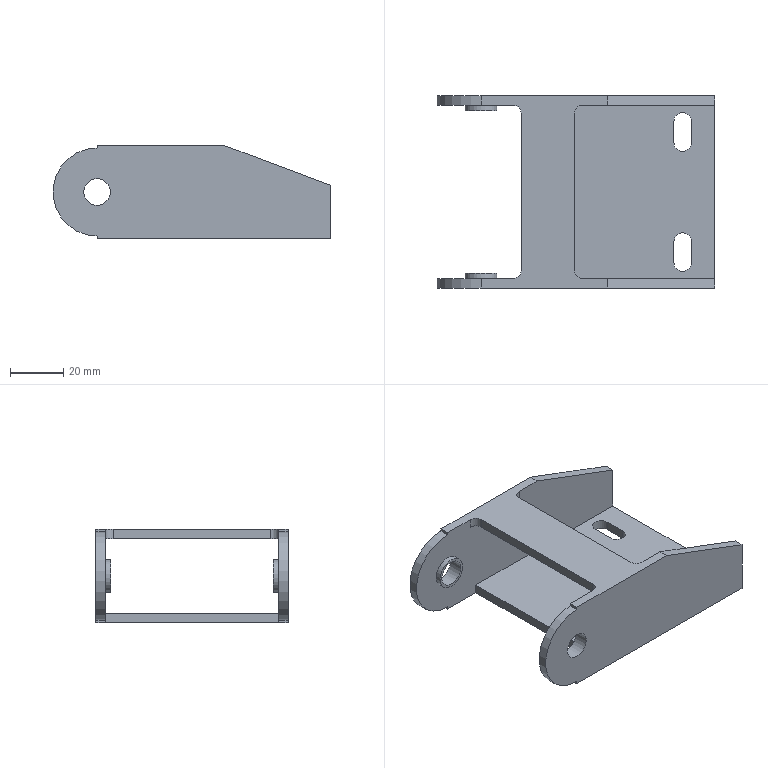Part | STEP file | 1 solid | 38 faces | box 104 x 72 x 35 mm | volume 42394 mm3 | plane 24 | cylinder 14 | commonest cylinder face diameters 6 x4 6.5 x4 10 x2 12 x2 33 x2